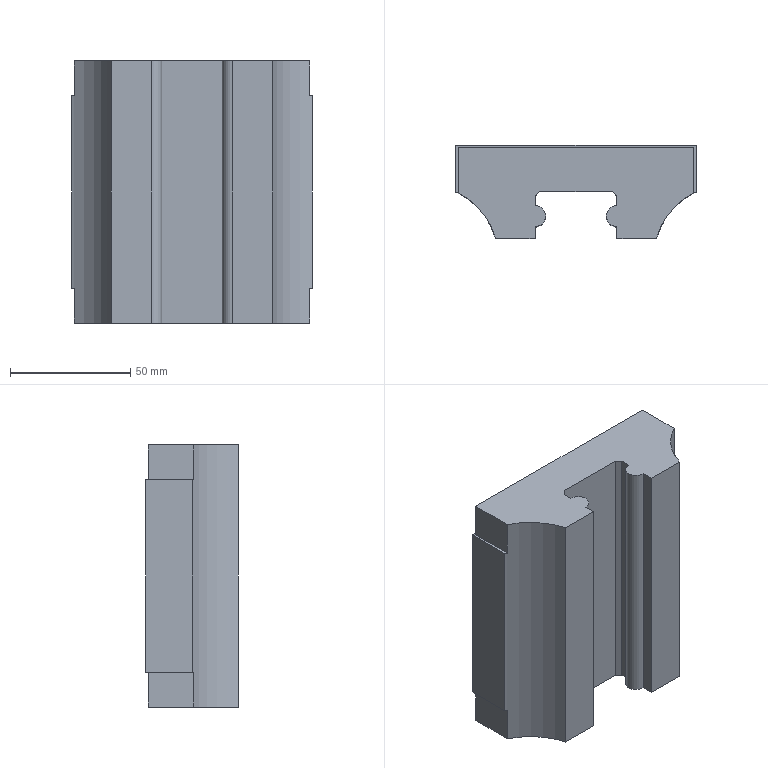Part | Creo | features CURVE 3, DATUM PLANE 3, PROTRUSION 2, COORDINATE SYSTEM 1, CUT 1 | 1 solid | 38 faces | box 100 x 38.5 x 109 mm | volume 303795 mm3 | plane 26 | cylinder 12 | commonest cylinder face diameters 6.8 x8 8.76 x2 59.72 x2
STEP:
#1=CARTESIAN_POINT('',(0.,0.,0.));
#2=DIRECTION('',(0.,0.,1.));
#3=DIRECTION('',(1.,0.,0.));
#4=AXIS2_PLACEMENT_3D('',#1,#2,#3);
#5=CARTESIAN_POINT('',(49.,37.5,-40.));
#6=VERTEX_POINT('',#5);
#7=CARTESIAN_POINT('',(-49.,37.5,-40.));
#8=VERTEX_POINT('',#7);
#9=CARTESIAN_POINT('',(49.,37.5,-40.));
#10=DIRECTION('',(-1.,0.,0.));
#11=VECTOR('',#10,98.);
#12=LINE('',#9,#11);
#13=EDGE_CURVE('',#6,#8,#12,.T.);
#14=ORIENTED_EDGE('',*,*,#13,.F.);
#15=CARTESIAN_POINT('',(49.,18.776,-40.));
#16=VERTEX_POINT('',#15);
#17=CARTESIAN_POINT('',(49.,18.776,-40.));
#18=DIRECTION('',(0.,1.,0.));
#19=VECTOR('',#18,18.724);
#20=LINE('',#17,#19);
#21=EDGE_CURVE('',#16,#6,#20,.T.);
#22=ORIENTED_EDGE('',*,*,#21,.F.);
#23=CARTESIAN_POINT('',(50.,19.25,-40.));
#24=VERTEX_POINT('',#23);
#25=CARTESIAN_POINT('',(62.277,-7.969,-40.));
#26=DIRECTION('',(0.,0.,-1.));
#27=DIRECTION('',(-0.4446,0.8957,0.));
#28=AXIS2_PLACEMENT_3D('',#25,#26,#27);
#29=CIRCLE('',#28,29.86);
#30=EDGE_CURVE('',#16,#24,#29,.T.);
#31=ORIENTED_EDGE('',*,*,#30,.T.);
#32=CARTESIAN_POINT('',(50.,38.5,-40.));
#33=VERTEX_POINT('',#32);
#34=CARTESIAN_POINT('',(50.,19.25,-40.));
#35=DIRECTION('',(0.,1.,0.));
#36=VECTOR('',#35,19.25);
#37=LINE('',#34,#36);
#38=EDGE_CURVE('',#24,#33,#37,.T.);
#39=ORIENTED_EDGE('',*,*,#38,.T.);
#40=CARTESIAN_POINT('',(-50.,38.5,-40.));
#41=VERTEX_POINT('',#40);
#42=CARTESIAN_POINT('',(50.,38.5,-40.));
#43=DIRECTION('',(-1.,0.,0.));
#44=VECTOR('',#43,100.);
#45=LINE('',#42,#44);
#46=EDGE_CURVE('',#33,#41,#45,.T.);
#47=ORIENTED_EDGE('',*,*,#46,.T.);
#48=CARTESIAN_POINT('',(-50.,19.25,-40.));
#49=VERTEX_POINT('',#48);
#50=CARTESIAN_POINT('',(-50.,38.5,-40.));
#51=DIRECTION('',(0.,-1.,0.));
#52=VECTOR('',#51,19.25);
#53=LINE('',#50,#52);
#54=EDGE_CURVE('',#41,#49,#53,.T.);
#55=ORIENTED_EDGE('',*,*,#54,.T.);
#56=CARTESIAN_POINT('',(-49.,18.776,-40.));
#57=VERTEX_POINT('',#56);
#58=CARTESIAN_POINT('',(-62.277,-7.969,-40.));
#59=DIRECTION('',(0.,0.,-1.));
#60=DIRECTION('',(0.4111,0.9116,0.));
#61=AXIS2_PLACEMENT_3D('',#58,#59,#60);
#62=CIRCLE('',#61,29.86);
#63=EDGE_CURVE('',#49,#57,#62,.T.);
#64=ORIENTED_EDGE('',*,*,#63,.T.);
#65=CARTESIAN_POINT('',(-49.,37.5,-40.));
#66=DIRECTION('',(0.,-1.,0.));
#67=VECTOR('',#66,18.724);
#68=LINE('',#65,#67);
#69=EDGE_CURVE('',#8,#57,#68,.T.);
#70=ORIENTED_EDGE('',*,*,#69,.F.);
#71=EDGE_LOOP('',(#14,#22,#31,#39,#47,#55,#64,#70));
#72=FACE_OUTER_BOUND('',#71,.F.);
#73=CARTESIAN_POINT('',(0.,0.,-40.));
#74=DIRECTION('',(0.,0.,1.));
#75=DIRECTION('',(1.,0.,0.));
#76=AXIS2_PLACEMENT_3D('',#73,#74,#75);
#77=PLANE('',#76);
#78=ADVANCED_FACE('',(#72),#77,.F.);
#79=ORIENTED_EDGE('',*,*,#13,.T.);
#80=CARTESIAN_POINT('',(-49.,37.5,-54.5));
#81=VERTEX_POINT('',#80);
#82=CARTESIAN_POINT('',(-49.,37.5,-54.5));
#83=DIRECTION('',(0.,0.,1.));
#84=VECTOR('',#83,14.5);
#85=LINE('',#82,#84);
#86=EDGE_CURVE('',#81,#8,#85,.T.);
#87=ORIENTED_EDGE('',*,*,#86,.F.);
#88=CARTESIAN_POINT('',(49.,37.5,-54.5));
#89=VERTEX_POINT('',#88);
#90=CARTESIAN_POINT('',(49.,37.5,-54.5));
#91=DIRECTION('',(-1.,0.,0.));
#92=VECTOR('',#91,98.);
#93=LINE('',#90,#92);
#94=EDGE_CURVE('',#89,#81,#93,.T.);
#95=ORIENTED_EDGE('',*,*,#94,.F.);
#96=CARTESIAN_POINT('',(49.,37.5,-54.5));
#97=DIRECTION('',(0.,0.,1.));
#98=VECTOR('',#97,14.5);
#99=LINE('',#96,#98);
#100=EDGE_CURVE('',#89,#6,#99,.T.);
#101=ORIENTED_EDGE('',*,*,#100,.T.);
#102=EDGE_LOOP('',(#79,#87,#95,#101));
#103=FACE_OUTER_BOUND('',#102,.F.);
#104=CARTESIAN_POINT('',(49.,37.5,-54.5));
#105=DIRECTION('',(0.,1.,0.));
#106=DIRECTION('',(-1.,0.,0.));
#107=AXIS2_PLACEMENT_3D('',#104,#105,#106);
#108=PLANE('',#107);
#109=ADVANCED_FACE('',(#103),#108,.T.);
#110=CARTESIAN_POINT('',(49.,37.5,40.));
#111=VERTEX_POINT('',#110);
#112=CARTESIAN_POINT('',(-49.,37.5,40.));
#113=VERTEX_POINT('',#112);
#114=CARTESIAN_POINT('',(49.,37.5,40.));
#115=DIRECTION('',(-1.,0.,0.));
#116=VECTOR('',#115,98.);
#117=LINE('',#114,#116);
#118=EDGE_CURVE('',#111,#113,#117,.T.);
#119=ORIENTED_EDGE('',*,*,#118,.F.);
#120=CARTESIAN_POINT('',(49.,37.5,54.5));
#121=VERTEX_POINT('',#120);
#122=CARTESIAN_POINT('',(49.,37.5,40.));
#123=DIRECTION('',(0.,0.,1.));
#124=VECTOR('',#123,14.5);
#125=LINE('',#122,#124);
#126=EDGE_CURVE('',#111,#121,#125,.T.);
#127=ORIENTED_EDGE('',*,*,#126,.T.);
#128=CARTESIAN_POINT('',(-49.,37.5,54.5));
#129=VERTEX_POINT('',#128);
#130=CARTESIAN_POINT('',(49.,37.5,54.5));
#131=DIRECTION('',(-1.,0.,0.));
#132=VECTOR('',#131,98.);
#133=LINE('',#130,#132);
#134=EDGE_CURVE('',#121,#129,#133,.T.);
#135=ORIENTED_EDGE('',*,*,#134,.T.);
#136=CARTESIAN_POINT('',(-49.,37.5,40.));
#137=DIRECTION('',(0.,0.,1.));
#138=VECTOR('',#137,14.5);
#139=LINE('',#136,#138);
#140=EDGE_CURVE('',#113,#129,#139,.T.);
#141=ORIENTED_EDGE('',*,*,#140,.F.);
#142=EDGE_LOOP('',(#119,#127,#135,#141));
#143=FACE_OUTER_BOUND('',#142,.F.);
#144=CARTESIAN_POINT('',(49.,37.5,-54.5));
#145=DIRECTION('',(0.,1.,0.));
#146=DIRECTION('',(-1.,0.,0.));
#147=AXIS2_PLACEMENT_3D('',#144,#145,#146);
#148=PLANE('',#147);
#149=ADVANCED_FACE('',(#143),#148,.T.);
#150=ORIENTED_EDGE('',*,*,#69,.T.);
#151=CARTESIAN_POINT('',(-49.,18.776,-54.5));
#152=VERTEX_POINT('',#151);
#153=CARTESIAN_POINT('',(-49.,18.776,-54.5));
#154=DIRECTION('',(0.,0.,1.));
#155=VECTOR('',#154,14.5);
#156=LINE('',#153,#155);
#157=EDGE_CURVE('',#152,#57,#156,.T.);
#158=ORIENTED_EDGE('',*,*,#157,.F.);
#159=CARTESIAN_POINT('',(-49.,37.5,-54.5));
#160=DIRECTION('',(0.,-1.,0.));
#161=VECTOR('',#160,18.724);
#162=LINE('',#159,#161);
#163=EDGE_CURVE('',#81,#152,#162,.T.);
#164=ORIENTED_EDGE('',*,*,#163,.F.);
#165=ORIENTED_EDGE('',*,*,#86,.T.);
#166=EDGE_LOOP('',(#150,#158,#164,#165));
#167=FACE_OUTER_BOUND('',#166,.F.);
#168=CARTESIAN_POINT('',(-49.,37.5,-54.5));
#169=DIRECTION('',(-1.,0.,0.));
#170=DIRECTION('',(0.,-1.,0.));
#171=AXIS2_PLACEMENT_3D('',#168,#169,#170);
#172=PLANE('',#171);
#173=ADVANCED_FACE('',(#167),#172,.T.);
#174=CARTESIAN_POINT('',(-49.,18.776,40.));
#175=VERTEX_POINT('',#174);
#176=CARTESIAN_POINT('',(-49.,37.5,40.));
#177=DIRECTION('',(0.,-1.,0.));
#178=VECTOR('',#177,18.724);
#179=LINE('',#176,#178);
#180=EDGE_CURVE('',#113,#175,#179,.T.);
#181=ORIENTED_EDGE('',*,*,#180,.F.);
#182=ORIENTED_EDGE('',*,*,#140,.T.);
#183=CARTESIAN_POINT('',(-49.,18.776,54.5));
#184=VERTEX_POINT('',#183);
#185=CARTESIAN_POINT('',(-49.,37.5,54.5));
#186=DIRECTION('',(0.,-1.,0.));
#187=VECTOR('',#186,18.724);
#188=LINE('',#185,#187);
#189=EDGE_CURVE('',#129,#184,#188,.T.);
#190=ORIENTED_EDGE('',*,*,#189,.T.);
#191=CARTESIAN_POINT('',(-49.,18.776,40.));
#192=DIRECTION('',(0.,0.,1.));
#193=VECTOR('',#192,14.5);
#194=LINE('',#191,#193);
#195=EDGE_CURVE('',#175,#184,#194,.T.);
#196=ORIENTED_EDGE('',*,*,#195,.F.);
#197=EDGE_LOOP('',(#181,#182,#190,#196));
#198=FACE_OUTER_BOUND('',#197,.F.);
#199=CARTESIAN_POINT('',(-49.,37.5,-54.5));
#200=DIRECTION('',(-1.,0.,0.));
#201=DIRECTION('',(0.,-1.,0.));
#202=AXIS2_PLACEMENT_3D('',#199,#200,#201);
#203=PLANE('',#202);
#204=ADVANCED_FACE('',(#198),#203,.T.);
#205=CARTESIAN_POINT('',(-50.,19.25,40.));
#206=VERTEX_POINT('',#205);
#207=CARTESIAN_POINT('',(-62.277,-7.969,40.));
#208=DIRECTION('',(0.,0.,-1.));
#209=DIRECTION('',(0.4111,0.9116,0.));
#210=AXIS2_PLACEMENT_3D('',#207,#208,#209);
#211=CIRCLE('',#210,29.86);
#212=EDGE_CURVE('',#206,#175,#211,.T.);
#213=ORIENTED_EDGE('',*,*,#212,.T.);
#214=ORIENTED_EDGE('',*,*,#195,.T.);
#215=CARTESIAN_POINT('',(-33.5,0.,54.5));
#216=VERTEX_POINT('',#215);
#217=CARTESIAN_POINT('',(-62.277,-7.969,54.5));
#218=DIRECTION('',(0.,0.,-1.));
#219=DIRECTION('',(0.4446,0.8957,0.));
#220=AXIS2_PLACEMENT_3D('',#217,#218,#219);
#221=CIRCLE('',#220,29.86);
#222=EDGE_CURVE('',#184,#216,#221,.T.);
#223=ORIENTED_EDGE('',*,*,#222,.T.);
#224=CARTESIAN_POINT('',(-33.5,0.,-54.5));
#225=VERTEX_POINT('',#224);
#226=CARTESIAN_POINT('',(-33.5,0.,-54.5));
#227=DIRECTION('',(0.,0.,1.));
#228=VECTOR('',#227,109.);
#229=LINE('',#226,#228);
#230=EDGE_CURVE('',#225,#216,#229,.T.);
#231=ORIENTED_EDGE('',*,*,#230,.F.);
#232=CARTESIAN_POINT('',(-62.277,-7.969,-54.5));
#233=DIRECTION('',(0.,0.,-1.));
#234=DIRECTION('',(0.4446,0.8957,0.));
#235=AXIS2_PLACEMENT_3D('',#232,#233,#234);
#236=CIRCLE('',#235,29.86);
#237=EDGE_CURVE('',#152,#225,#236,.T.);
#238=ORIENTED_EDGE('',*,*,#237,.F.);
#239=ORIENTED_EDGE('',*,*,#157,.T.);
#240=ORIENTED_EDGE('',*,*,#63,.F.);
#241=CARTESIAN_POINT('',(-50.,19.25,-40.));
#242=DIRECTION('',(0.,0.,1.));
#243=VECTOR('',#242,80.);
#244=LINE('',#241,#243);
#245=EDGE_CURVE('',#49,#206,#244,.T.);
#246=ORIENTED_EDGE('',*,*,#245,.T.);
#247=EDGE_LOOP('',(#213,#214,#223,#231,#238,#239,#240,#246));
#248=FACE_OUTER_BOUND('',#247,.F.);
#249=CARTESIAN_POINT('',(-62.277,-7.969,-40.));
#250=DIRECTION('',(0.,0.,1.));
#251=DIRECTION('',(1.,0.,0.));
#252=AXIS2_PLACEMENT_3D('',#249,#250,#251);
#253=CYLINDRICAL_SURFACE('',#252,29.86);
#254=ADVANCED_FACE('',(#248),#253,.F.);
#255=ORIENTED_EDGE('',*,*,#118,.T.);
#256=ORIENTED_EDGE('',*,*,#180,.T.);
#257=ORIENTED_EDGE('',*,*,#212,.F.);
#258=CARTESIAN_POINT('',(-50.,38.5,40.));
#259=VERTEX_POINT('',#258);
#260=CARTESIAN_POINT('',(-50.,38.5,40.));
#261=DIRECTION('',(0.,-1.,0.));
#262=VECTOR('',#261,19.25);
#263=LINE('',#260,#262);
#264=EDGE_CURVE('',#259,#206,#263,.T.);
#265=ORIENTED_EDGE('',*,*,#264,.F.);
#266=CARTESIAN_POINT('',(50.,38.5,40.));
#267=VERTEX_POINT('',#266);
#268=CARTESIAN_POINT('',(50.,38.5,40.));
#269=DIRECTION('',(-1.,0.,0.));
#270=VECTOR('',#269,100.);
#271=LINE('',#268,#270);
#272=EDGE_CURVE('',#267,#259,#271,.T.);
#273=ORIENTED_EDGE('',*,*,#272,.F.);
#274=CARTESIAN_POINT('',(50.,19.25,40.));
#275=VERTEX_POINT('',#274);
#276=CARTESIAN_POINT('',(50.,19.25,40.));
#277=DIRECTION('',(0.,1.,0.));
#278=VECTOR('',#277,19.25);
#279=LINE('',#276,#278);
#280=EDGE_CURVE('',#275,#267,#279,.T.);
#281=ORIENTED_EDGE('',*,*,#280,.F.);
#282=CARTESIAN_POINT('',(49.,18.776,40.));
#283=VERTEX_POINT('',#282);
#284=CARTESIAN_POINT('',(62.277,-7.969,40.));
#285=DIRECTION('',(0.,0.,-1.));
#286=DIRECTION('',(-0.4446,0.8957,0.));
#287=AXIS2_PLACEMENT_3D('',#284,#285,#286);
#288=CIRCLE('',#287,29.86);
#289=EDGE_CURVE('',#283,#275,#288,.T.);
#290=ORIENTED_EDGE('',*,*,#289,.F.);
#291=CARTESIAN_POINT('',(49.,18.776,40.));
#292=DIRECTION('',(0.,1.,0.));
#293=VECTOR('',#292,18.724);
#294=LINE('',#291,#293);
#295=EDGE_CURVE('',#283,#111,#294,.T.);
#296=ORIENTED_EDGE('',*,*,#295,.T.);
#297=EDGE_LOOP('',(#255,#256,#257,#265,#273,#281,#290,#296));
#298=FACE_OUTER_BOUND('',#297,.F.);
#299=CARTESIAN_POINT('',(0.,0.,40.));
#300=DIRECTION('',(0.,0.,1.));
#301=DIRECTION('',(1.,0.,0.));
#302=AXIS2_PLACEMENT_3D('',#299,#300,#301);
#303=PLANE('',#302);
#304=ADVANCED_FACE('',(#298),#303,.T.);
#305=ORIENTED_EDGE('',*,*,#54,.F.);
#306=CARTESIAN_POINT('',(-50.,38.5,-40.));
#307=DIRECTION('',(0.,0.,1.));
#308=VECTOR('',#307,80.);
#309=LINE('',#306,#308);
#310=EDGE_CURVE('',#41,#259,#309,.T.);
#311=ORIENTED_EDGE('',*,*,#310,.T.);
#312=ORIENTED_EDGE('',*,*,#264,.T.);
#313=ORIENTED_EDGE('',*,*,#245,.F.);
#314=EDGE_LOOP('',(#305,#311,#312,#313));
#315=FACE_OUTER_BOUND('',#314,.F.);
#316=CARTESIAN_POINT('',(-50.,38.5,-40.));
#317=DIRECTION('',(-1.,0.,0.));
#318=DIRECTION('',(0.,-1.,0.));
#319=AXIS2_PLACEMENT_3D('',#316,#317,#318);
#320=PLANE('',#319);
#321=ADVANCED_FACE('',(#315),#320,.T.);
#322=ORIENTED_EDGE('',*,*,#46,.F.);
#323=CARTESIAN_POINT('',(50.,38.5,-40.));
#324=DIRECTION('',(0.,0.,1.));
#325=VECTOR('',#324,80.);
#326=LINE('',#323,#325);
#327=EDGE_CURVE('',#33,#267,#326,.T.);
#328=ORIENTED_EDGE('',*,*,#327,.T.);
#329=ORIENTED_EDGE('',*,*,#272,.T.);
#330=ORIENTED_EDGE('',*,*,#310,.F.);
#331=EDGE_LOOP('',(#322,#328,#329,#330));
#332=FACE_OUTER_BOUND('',#331,.F.);
#333=CARTESIAN_POINT('',(44.4,38.5,-31.));
#334=VERTEX_POINT('',#333);
#335=CARTESIAN_POINT('',(37.6,38.5,-31.));
#336=VERTEX_POINT('',#335);
#337=CARTESIAN_POINT('',(41.,38.5,-31.));
#338=DIRECTION('',(0.,1.,0.));
#339=DIRECTION('',(1.,0.,0.));
#340=AXIS2_PLACEMENT_3D('',#337,#338,#339);
#341=CIRCLE('',#340,3.4);
#342=EDGE_CURVE('',#334,#336,#341,.T.);
#343=ORIENTED_EDGE('',*,*,#342,.T.);
#344=CARTESIAN_POINT('',(41.,38.5,-31.));
#345=DIRECTION('',(0.,1.,0.));
#346=DIRECTION('',(-1.,0.,0.));
#347=AXIS2_PLACEMENT_3D('',#344,#345,#346);
#348=CIRCLE('',#347,3.4);
#349=EDGE_CURVE('',#336,#334,#348,.T.);
#350=ORIENTED_EDGE('',*,*,#349,.T.);
#351=EDGE_LOOP('',(#343,#350));
#352=FACE_BOUND('',#351,.F.);
#353=CARTESIAN_POINT('',(-37.6,38.5,-31.));
#354=VERTEX_POINT('',#353);
#355=CARTESIAN_POINT('',(-44.4,38.5,-31.));
#356=VERTEX_POINT('',#355);
#357=CARTESIAN_POINT('',(-41.,38.5,-31.));
#358=DIRECTION('',(0.,1.,0.));
#359=DIRECTION('',(1.,0.,0.));
#360=AXIS2_PLACEMENT_3D('',#357,#358,#359);
#361=CIRCLE('',#360,3.4);
#362=EDGE_CURVE('',#354,#356,#361,.T.);
#363=ORIENTED_EDGE('',*,*,#362,.T.);
#364=CARTESIAN_POINT('',(-41.,38.5,-31.));
#365=DIRECTION('',(0.,1.,0.));
#366=DIRECTION('',(-1.,0.,0.));
#367=AXIS2_PLACEMENT_3D('',#364,#365,#366);
#368=CIRCLE('',#367,3.4);
#369=EDGE_CURVE('',#356,#354,#368,.T.);
#370=ORIENTED_EDGE('',*,*,#369,.T.);
#371=EDGE_LOOP('',(#363,#370));
#372=FACE_BOUND('',#371,.F.);
#373=CARTESIAN_POINT('',(-37.6,38.5,31.));
#374=VERTEX_POINT('',#373);
#375=CARTESIAN_POINT('',(-44.4,38.5,31.));
#376=VERTEX_POINT('',#375);
#377=CARTESIAN_POINT('',(-41.,38.5,31.));
#378=DIRECTION('',(0.,1.,0.));
#379=DIRECTION('',(1.,0.,0.));
#380=AXIS2_PLACEMENT_3D('',#377,#378,#379);
#381=CIRCLE('',#380,3.4);
#382=EDGE_CURVE('',#374,#376,#381,.T.);
#383=ORIENTED_EDGE('',*,*,#382,.T.);
#384=CARTESIAN_POINT('',(-41.,38.5,31.));
#385=DIRECTION('',(0.,1.,0.));
#386=DIRECTION('',(-1.,0.,0.));
#387=AXIS2_PLACEMENT_3D('',#384,#385,#386);
#388=CIRCLE('',#387,3.4);
#389=EDGE_CURVE('',#376,#374,#388,.T.);
#390=ORIENTED_EDGE('',*,*,#389,.T.);
#391=EDGE_LOOP('',(#383,#390));
#392=FACE_BOUND('',#391,.F.);
#393=CARTESIAN_POINT('',(44.4,38.5,31.));
#394=VERTEX_POINT('',#393);
#395=CARTESIAN_POINT('',(37.6,38.5,31.));
#396=VERTEX_POINT('',#395);
#397=CARTESIAN_POINT('',(41.,38.5,31.));
#398=DIRECTION('',(0.,1.,0.));
#399=DIRECTION('',(1.,0.,0.));
#400=AXIS2_PLACEMENT_3D('',#397,#398,#399);
#401=CIRCLE('',#400,3.4);
#402=EDGE_CURVE('',#394,#396,#401,.T.);
#403=ORIENTED_EDGE('',*,*,#402,.T.);
#404=CARTESIAN_POINT('',(41.,38.5,31.));
#405=DIRECTION('',(0.,1.,0.));
#406=DIRECTION('',(-1.,0.,0.));
#407=AXIS2_PLACEMENT_3D('',#404,#405,#406);
#408=CIRCLE('',#407,3.4);
#409=EDGE_CURVE('',#396,#394,#408,.T.);
#410=ORIENTED_EDGE('',*,*,#409,.T.);
#411=EDGE_LOOP('',(#403,#410));
#412=FACE_BOUND('',#411,.F.);
#413=CARTESIAN_POINT('',(50.,38.5,-40.));
#414=DIRECTION('',(0.,1.,0.));
#415=DIRECTION('',(-1.,0.,0.));
#416=AXIS2_PLACEMENT_3D('',#413,#414,#415);
#417=PLANE('',#416);
#418=ADVANCED_FACE('',(#332,#352,#372,#392,#412),#417,.T.);
#419=ORIENTED_EDGE('',*,*,#38,.F.);
#420=CARTESIAN_POINT('',(50.,19.25,-40.));
#421=DIRECTION('',(0.,0.,1.));
#422=VECTOR('',#421,80.);
#423=LINE('',#420,#422);
#424=EDGE_CURVE('',#24,#275,#423,.T.);
#425=ORIENTED_EDGE('',*,*,#424,.T.);
#426=ORIENTED_EDGE('',*,*,#280,.T.);
#427=ORIENTED_EDGE('',*,*,#327,.F.);
#428=EDGE_LOOP('',(#419,#425,#426,#427));
#429=FACE_OUTER_BOUND('',#428,.F.);
#430=CARTESIAN_POINT('',(50.,19.25,-40.));
#431=DIRECTION('',(1.,0.,0.));
#432=DIRECTION('',(0.,1.,0.));
#433=AXIS2_PLACEMENT_3D('',#430,#431,#432);
#434=PLANE('',#433);
#435=ADVANCED_FACE('',(#429),#434,.T.);
#436=CARTESIAN_POINT('',(33.5,0.,-54.5));
#437=VERTEX_POINT('',#436);
#438=CARTESIAN_POINT('',(33.5,0.,54.5));
#439=VERTEX_POINT('',#438);
#440=CARTESIAN_POINT('',(33.5,0.,-54.5));
#441=DIRECTION('',(0.,0.,1.));
#442=VECTOR('',#441,109.);
#443=LINE('',#440,#442);
#444=EDGE_CURVE('',#437,#439,#443,.T.);
#445=ORIENTED_EDGE('',*,*,#444,.T.);
#446=CARTESIAN_POINT('',(49.,18.776,54.5));
#447=VERTEX_POINT('',#446);
#448=CARTESIAN_POINT('',(62.277,-7.969,54.5));
#449=DIRECTION('',(0.,0.,-1.));
#450=DIRECTION('',(-0.9637,0.2669,0.));
#451=AXIS2_PLACEMENT_3D('',#448,#449,#450);
#452=CIRCLE('',#451,29.86);
#453=EDGE_CURVE('',#439,#447,#452,.T.);
#454=ORIENTED_EDGE('',*,*,#453,.T.);
#455=CARTESIAN_POINT('',(49.,18.776,40.));
#456=DIRECTION('',(0.,0.,1.));
#457=VECTOR('',#456,14.5);
#458=LINE('',#455,#457);
#459=EDGE_CURVE('',#283,#447,#458,.T.);
#460=ORIENTED_EDGE('',*,*,#459,.F.);
#461=ORIENTED_EDGE('',*,*,#289,.T.);
#462=ORIENTED_EDGE('',*,*,#424,.F.);
#463=ORIENTED_EDGE('',*,*,#30,.F.);
#464=CARTESIAN_POINT('',(49.,18.776,-54.5));
#465=VERTEX_POINT('',#464);
#466=CARTESIAN_POINT('',(49.,18.776,-54.5));
#467=DIRECTION('',(0.,0.,1.));
#468=VECTOR('',#467,14.5);
#469=LINE('',#466,#468);
#470=EDGE_CURVE('',#465,#16,#469,.T.);
#471=ORIENTED_EDGE('',*,*,#470,.F.);
#472=CARTESIAN_POINT('',(62.277,-7.969,-54.5));
#473=DIRECTION('',(0.,0.,-1.));
#474=DIRECTION('',(-0.9637,0.2669,0.));
#475=AXIS2_PLACEMENT_3D('',#472,#473,#474);
#476=CIRCLE('',#475,29.86);
#477=EDGE_CURVE('',#437,#465,#476,.T.);
#478=ORIENTED_EDGE('',*,*,#477,.F.);
#479=EDGE_LOOP('',(#445,#454,#460,#461,#462,#463,#471,#478));
#480=FACE_OUTER_BOUND('',#479,.F.);
#481=CARTESIAN_POINT('',(62.277,-7.969,-40.));
#482=DIRECTION('',(0.,0.,1.));
#483=DIRECTION('',(1.,0.,0.));
#484=AXIS2_PLACEMENT_3D('',#481,#482,#483);
#485=CYLINDRICAL_SURFACE('',#484,29.86);
#486=ADVANCED_FACE('',(#480),#485,.F.);
#487=CARTESIAN_POINT('',(17.,0.,-54.5));
#488=VERTEX_POINT('',#487);
#489=CARTESIAN_POINT('',(17.,0.,54.5));
#490=VERTEX_POINT('',#489);
#491=CARTESIAN_POINT('',(17.,0.,-54.5));
#492=DIRECTION('',(0.,0.,1.));
#493=VECTOR('',#492,109.);
#494=LINE('',#491,#493);
#495=EDGE_CURVE('',#488,#490,#494,.T.);
#496=ORIENTED_EDGE('',*,*,#495,.T.);
#497=CARTESIAN_POINT('',(17.,0.,54.5));
#498=DIRECTION('',(1.,0.,0.));
#499=VECTOR('',#498,16.5);
#500=LINE('',#497,#499);
#501=EDGE_CURVE('',#490,#439,#500,.T.);
#502=ORIENTED_EDGE('',*,*,#501,.T.);
#503=ORIENTED_EDGE('',*,*,#444,.F.);
#504=CARTESIAN_POINT('',(17.,0.,-54.5));
#505=DIRECTION('',(1.,0.,0.));
#506=VECTOR('',#505,16.5);
#507=LINE('',#504,#506);
#508=EDGE_CURVE('',#488,#437,#507,.T.);
#509=ORIENTED_EDGE('',*,*,#508,.F.);
#510=EDGE_LOOP('',(#496,#502,#503,#509));
#511=FACE_OUTER_BOUND('',#510,.F.);
#512=CARTESIAN_POINT('',(17.,0.,-40.));
#513=DIRECTION('',(0.,-1.,0.));
#514=DIRECTION('',(1.,0.,0.));
#515=AXIS2_PLACEMENT_3D('',#512,#513,#514);
#516=PLANE('',#515);
#517=ADVANCED_FACE('',(#511),#516,.T.);
#518=CARTESIAN_POINT('',(17.,4.72,-54.5));
#519=VERTEX_POINT('',#518);
#520=CARTESIAN_POINT('',(17.,4.72,54.5));
#521=VERTEX_POINT('',#520);
#522=CARTESIAN_POINT('',(17.,4.72,-54.5));
#523=DIRECTION('',(0.,0.,1.));
#524=VECTOR('',#523,109.);
#525=LINE('',#522,#524);
#526=EDGE_CURVE('',#519,#521,#525,.T.);
#527=ORIENTED_EDGE('',*,*,#526,.T.);
#528=CARTESIAN_POINT('',(17.,4.72,54.5));
#529=DIRECTION('',(0.,-1.,0.));
#530=VECTOR('',#529,4.72);
#531=LINE('',#528,#530);
#532=EDGE_CURVE('',#521,#490,#531,.T.);
#533=ORIENTED_EDGE('',*,*,#532,.T.);
#534=ORIENTED_EDGE('',*,*,#495,.F.);
#535=CARTESIAN_POINT('',(17.,4.72,-54.5));
#536=DIRECTION('',(0.,-1.,0.));
#537=VECTOR('',#536,4.72);
#538=LINE('',#535,#537);
#539=EDGE_CURVE('',#519,#488,#538,.T.);
#540=ORIENTED_EDGE('',*,*,#539,.F.);
#541=EDGE_LOOP('',(#527,#533,#534,#540));
#542=FACE_OUTER_BOUND('',#541,.F.);
#543=CARTESIAN_POINT('',(17.,4.72,-40.));
#544=DIRECTION('',(-1.,0.,0.));
#545=DIRECTION('',(0.,-1.,0.));
#546=AXIS2_PLACEMENT_3D('',#543,#544,#545);
#547=PLANE('',#546);
#548=ADVANCED_FACE('',(#542),#547,.T.);
#549=CARTESIAN_POINT('',(17.,13.48,-54.5));
#550=VERTEX_POINT('',#549);
#551=CARTESIAN_POINT('',(17.,13.48,54.5));
#552=VERTEX_POINT('',#551);
#553=CARTESIAN_POINT('',(17.,13.48,-54.5));
#554=DIRECTION('',(0.,0.,1.));
#555=VECTOR('',#554,109.);
#556=LINE('',#553,#555);
#557=EDGE_CURVE('',#550,#552,#556,.T.);
#558=ORIENTED_EDGE('',*,*,#557,.T.);
#559=CARTESIAN_POINT('',(17.,9.1,54.5));
#560=DIRECTION('',(0.,0.,1.));
#561=DIRECTION('',(0.,1.,0.));
#562=AXIS2_PLACEMENT_3D('',#559,#560,#561);
#563=CIRCLE('',#562,4.38);
#564=EDGE_CURVE('',#552,#521,#563,.T.);
#565=ORIENTED_EDGE('',*,*,#564,.T.);
#566=ORIENTED_EDGE('',*,*,#526,.F.);
#567=CARTESIAN_POINT('',(17.,9.1,-54.5));
#568=DIRECTION('',(0.,0.,1.));
#569=DIRECTION('',(0.,1.,0.));
#570=AXIS2_PLACEMENT_3D('',#567,#568,#569);
#571=CIRCLE('',#570,4.38);
#572=EDGE_CURVE('',#550,#519,#571,.T.);
#573=ORIENTED_EDGE('',*,*,#572,.F.);
#574=EDGE_LOOP('',(#558,#565,#566,#573));
#575=FACE_OUTER_BOUND('',#574,.F.);
#576=CARTESIAN_POINT('',(17.,9.1,-40.));
#577=DIRECTION('',(0.,0.,1.));
#578=DIRECTION('',(1.,0.,0.));
#579=AXIS2_PLACEMENT_3D('',#576,#577,#578);
#580=CYLINDRICAL_SURFACE('',#579,4.38);
#581=ADVANCED_FACE('',(#575),#580,.T.);
#582=CARTESIAN_POINT('',(17.,17.51,-54.5));
#583=VERTEX_POINT('',#582);
#584=CARTESIAN_POINT('',(17.,17.51,54.5));
#585=VERTEX_POINT('',#584);
#586=CARTESIAN_POINT('',(17.,17.51,-54.5));
#587=DIRECTION('',(0.,0.,1.));
#588=VECTOR('',#587,109.);
#589=LINE('',#586,#588);
#590=EDGE_CURVE('',#583,#585,#589,.T.);
#591=ORIENTED_EDGE('',*,*,#590,.T.);
#592=CARTESIAN_POINT('',(17.,17.51,54.5));
#593=DIRECTION('',(0.,-1.,0.));
#594=VECTOR('',#593,4.03);
#595=LINE('',#592,#594);
#596=EDGE_CURVE('',#585,#552,#595,.T.);
#597=ORIENTED_EDGE('',*,*,#596,.T.);
#598=ORIENTED_EDGE('',*,*,#557,.F.);
#599=CARTESIAN_POINT('',(17.,17.51,-54.5));
#600=DIRECTION('',(0.,-1.,0.));
#601=VECTOR('',#600,4.03);
#602=LINE('',#599,#601);
#603=EDGE_CURVE('',#583,#550,#602,.T.);
#604=ORIENTED_EDGE('',*,*,#603,.F.);
#605=EDGE_LOOP('',(#591,#597,#598,#604));
#606=FACE_OUTER_BOUND('',#605,.F.);
#607=CARTESIAN_POINT('',(17.,17.51,-40.));
#608=DIRECTION('',(-1.,0.,0.));
#609=DIRECTION('',(0.,-1.,0.));
#610=AXIS2_PLACEMENT_3D('',#607,#608,#609);
#611=PLANE('',#610);
#612=ADVANCED_FACE('',(#606),#611,.T.);
#613=CARTESIAN_POINT('',(15.,19.51,-54.5));
#614=VERTEX_POINT('',#613);
#615=CARTESIAN_POINT('',(15.,19.51,54.5));
#616=VERTEX_POINT('',#615);
#617=CARTESIAN_POINT('',(15.,19.51,-54.5));
#618=DIRECTION('',(0.,0.,1.));
#619=VECTOR('',#618,109.);
#620=LINE('',#617,#619);
#621=EDGE_CURVE('',#614,#616,#620,.T.);
#622=ORIENTED_EDGE('',*,*,#621,.T.);
#623=CARTESIAN_POINT('',(15.,19.51,54.5));
#624=DIRECTION('',(0.7071,-0.7071,0.));
#625=VECTOR('',#624,2.828);
#626=LINE('',#623,#625);
#627=EDGE_CURVE('',#616,#585,#626,.T.);
#628=ORIENTED_EDGE('',*,*,#627,.T.);
#629=ORIENTED_EDGE('',*,*,#590,.F.);
#630=CARTESIAN_POINT('',(15.,19.51,-54.5));
#631=DIRECTION('',(0.7071,-0.7071,0.));
#632=VECTOR('',#631,2.828);
#633=LINE('',#630,#632);
#634=EDGE_CURVE('',#614,#583,#633,.T.);
#635=ORIENTED_EDGE('',*,*,#634,.F.);
#636=EDGE_LOOP('',(#622,#628,#629,#635));
#637=FACE_OUTER_BOUND('',#636,.F.);
#638=CARTESIAN_POINT('',(15.,19.51,-40.));
#639=DIRECTION('',(-0.7071,-0.7071,0.));
#640=DIRECTION('',(0.7071,-0.7071,0.));
#641=AXIS2_PLACEMENT_3D('',#638,#639,#640);
#642=PLANE('',#641);
#643=ADVANCED_FACE('',(#637),#642,.T.);
#644=CARTESIAN_POINT('',(-15.,19.51,-54.5));
#645=VERTEX_POINT('',#644);
#646=CARTESIAN_POINT('',(-15.,19.51,54.5));
#647=VERTEX_POINT('',#646);
#648=CARTESIAN_POINT('',(-15.,19.51,-54.5));
#649=DIRECTION('',(0.,0.,1.));
#650=VECTOR('',#649,109.);
#651=LINE('',#648,#650);
#652=EDGE_CURVE('',#645,#647,#651,.T.);
#653=ORIENTED_EDGE('',*,*,#652,.T.);
#654=CARTESIAN_POINT('',(-15.,19.51,54.5));
#655=DIRECTION('',(1.,0.,0.));
#656=VECTOR('',#655,30.);
#657=LINE('',#654,#656);
#658=EDGE_CURVE('',#647,#616,#657,.T.);
#659=ORIENTED_EDGE('',*,*,#658,.T.);
#660=ORIENTED_EDGE('',*,*,#621,.F.);
#661=CARTESIAN_POINT('',(-15.,19.51,-54.5));
#662=DIRECTION('',(1.,0.,0.));
#663=VECTOR('',#662,30.);
#664=LINE('',#661,#663);
#665=EDGE_CURVE('',#645,#614,#664,.T.);
#666=ORIENTED_EDGE('',*,*,#665,.F.);
#667=EDGE_LOOP('',(#653,#659,#660,#666));
#668=FACE_OUTER_BOUND('',#667,.F.);
#669=CARTESIAN_POINT('',(-15.,19.51,-40.));
#670=DIRECTION('',(0.,-1.,0.));
#671=DIRECTION('',(1.,0.,0.));
#672=AXIS2_PLACEMENT_3D('',#669,#670,#671);
#673=PLANE('',#672);
#674=ADVANCED_FACE('',(#668),#673,.T.);
#675=CARTESIAN_POINT('',(-17.,17.51,-54.5));
#676=VERTEX_POINT('',#675);
#677=CARTESIAN_POINT('',(-17.,17.51,54.5));
#678=VERTEX_POINT('',#677);
#679=CARTESIAN_POINT('',(-17.,17.51,-54.5));
#680=DIRECTION('',(0.,0.,1.));
#681=VECTOR('',#680,109.);
#682=LINE('',#679,#681);
#683=EDGE_CURVE('',#676,#678,#682,.T.);
#684=ORIENTED_EDGE('',*,*,#683,.T.);
#685=CARTESIAN_POINT('',(-17.,17.51,54.5));
#686=DIRECTION('',(0.7071,0.7071,0.));
#687=VECTOR('',#686,2.828);
#688=LINE('',#685,#687);
#689=EDGE_CURVE('',#678,#647,#688,.T.);
#690=ORIENTED_EDGE('',*,*,#689,.T.);
#691=ORIENTED_EDGE('',*,*,#652,.F.);
#692=CARTESIAN_POINT('',(-17.,17.51,-54.5));
#693=DIRECTION('',(0.7071,0.7071,0.));
#694=VECTOR('',#693,2.828);
#695=LINE('',#692,#694);
#696=EDGE_CURVE('',#676,#645,#695,.T.);
#697=ORIENTED_EDGE('',*,*,#696,.F.);
#698=EDGE_LOOP('',(#684,#690,#691,#697));
#699=FACE_OUTER_BOUND('',#698,.F.);
#700=CARTESIAN_POINT('',(-17.,17.51,-40.));
#701=DIRECTION('',(0.7071,-0.7071,0.));
#702=DIRECTION('',(0.7071,0.7071,0.));
#703=AXIS2_PLACEMENT_3D('',#700,#701,#702);
#704=PLANE('',#703);
#705=ADVANCED_FACE('',(#699),#704,.T.);
#706=CARTESIAN_POINT('',(-17.,13.48,-54.5));
#707=VERTEX_POINT('',#706);
#708=CARTESIAN_POINT('',(-17.,13.48,54.5));
#709=VERTEX_POINT('',#708);
#710=CARTESIAN_POINT('',(-17.,13.48,-54.5));
#711=DIRECTION('',(0.,0.,1.));
#712=VECTOR('',#711,109.);
#713=LINE('',#710,#712);
#714=EDGE_CURVE('',#707,#709,#713,.T.);
#715=ORIENTED_EDGE('',*,*,#714,.T.);
#716=CARTESIAN_POINT('',(-17.,13.48,54.5));
#717=DIRECTION('',(0.,1.,0.));
#718=VECTOR('',#717,4.03);
#719=LINE('',#716,#718);
#720=EDGE_CURVE('',#709,#678,#719,.T.);
#721=ORIENTED_EDGE('',*,*,#720,.T.);
#722=ORIENTED_EDGE('',*,*,#683,.F.);
#723=CARTESIAN_POINT('',(-17.,13.48,-54.5));
#724=DIRECTION('',(0.,1.,0.));
#725=VECTOR('',#724,4.03);
#726=LINE('',#723,#725);
#727=EDGE_CURVE('',#707,#676,#726,.T.);
#728=ORIENTED_EDGE('',*,*,#727,.F.);
#729=EDGE_LOOP('',(#715,#721,#722,#728));
#730=FACE_OUTER_BOUND('',#729,.F.);
#731=CARTESIAN_POINT('',(-17.,13.48,-40.));
#732=DIRECTION('',(1.,0.,0.));
#733=DIRECTION('',(0.,1.,0.));
#734=AXIS2_PLACEMENT_3D('',#731,#732,#733);
#735=PLANE('',#734);
#736=ADVANCED_FACE('',(#730),#735,.T.);
#737=CARTESIAN_POINT('',(-17.,4.72,-54.5));
#738=VERTEX_POINT('',#737);
#739=CARTESIAN_POINT('',(-17.,4.72,54.5));
#740=VERTEX_POINT('',#739);
#741=CARTESIAN_POINT('',(-17.,4.72,-54.5));
#742=DIRECTION('',(0.,0.,1.));
#743=VECTOR('',#742,109.);
#744=LINE('',#741,#743);
#745=EDGE_CURVE('',#738,#740,#744,.T.);
#746=ORIENTED_EDGE('',*,*,#745,.T.);
#747=CARTESIAN_POINT('',(-17.,9.1,54.5));
#748=DIRECTION('',(0.,0.,1.));
#749=DIRECTION('',(0.,-1.,0.));
#750=AXIS2_PLACEMENT_3D('',#747,#748,#749);
#751=CIRCLE('',#750,4.38);
#752=EDGE_CURVE('',#740,#709,#751,.T.);
#753=ORIENTED_EDGE('',*,*,#752,.T.);
#754=ORIENTED_EDGE('',*,*,#714,.F.);
#755=CARTESIAN_POINT('',(-17.,9.1,-54.5));
#756=DIRECTION('',(0.,0.,1.));
#757=DIRECTION('',(0.,-1.,0.));
#758=AXIS2_PLACEMENT_3D('',#755,#756,#757);
#759=CIRCLE('',#758,4.38);
#760=EDGE_CURVE('',#738,#707,#759,.T.);
#761=ORIENTED_EDGE('',*,*,#760,.F.);
#762=EDGE_LOOP('',(#746,#753,#754,#761));
#763=FACE_OUTER_BOUND('',#762,.F.);
#764=CARTESIAN_POINT('',(-17.,9.1,-40.));
#765=DIRECTION('',(0.,0.,1.));
#766=DIRECTION('',(1.,0.,0.));
#767=AXIS2_PLACEMENT_3D('',#764,#765,#766);
#768=CYLINDRICAL_SURFACE('',#767,4.38);
#769=ADVANCED_FACE('',(#763),#768,.T.);
#770=CARTESIAN_POINT('',(-17.,0.,-54.5));
#771=VERTEX_POINT('',#770);
#772=CARTESIAN_POINT('',(-17.,0.,54.5));
#773=VERTEX_POINT('',#772);
#774=CARTESIAN_POINT('',(-17.,0.,-54.5));
#775=DIRECTION('',(0.,0.,1.));
#776=VECTOR('',#775,109.);
#777=LINE('',#774,#776);
#778=EDGE_CURVE('',#771,#773,#777,.T.);
#779=ORIENTED_EDGE('',*,*,#778,.T.);
#780=CARTESIAN_POINT('',(-17.,0.,54.5));
#781=DIRECTION('',(0.,1.,0.));
#782=VECTOR('',#781,4.72);
#783=LINE('',#780,#782);
#784=EDGE_CURVE('',#773,#740,#783,.T.);
#785=ORIENTED_EDGE('',*,*,#784,.T.);
#786=ORIENTED_EDGE('',*,*,#745,.F.);
#787=CARTESIAN_POINT('',(-17.,0.,-54.5));
#788=DIRECTION('',(0.,1.,0.));
#789=VECTOR('',#788,4.72);
#790=LINE('',#787,#789);
#791=EDGE_CURVE('',#771,#738,#790,.T.);
#792=ORIENTED_EDGE('',*,*,#791,.F.);
#793=EDGE_LOOP('',(#779,#785,#786,#792));
#794=FACE_OUTER_BOUND('',#793,.F.);
#795=CARTESIAN_POINT('',(-17.,0.,-40.));
#796=DIRECTION('',(1.,0.,0.));
#797=DIRECTION('',(0.,1.,0.));
#798=AXIS2_PLACEMENT_3D('',#795,#796,#797);
#799=PLANE('',#798);
#800=ADVANCED_FACE('',(#794),#799,.T.);
#801=ORIENTED_EDGE('',*,*,#230,.T.);
#802=CARTESIAN_POINT('',(-33.5,0.,54.5));
#803=DIRECTION('',(1.,0.,0.));
#804=VECTOR('',#803,16.5);
#805=LINE('',#802,#804);
#806=EDGE_CURVE('',#216,#773,#805,.T.);
#807=ORIENTED_EDGE('',*,*,#806,.T.);
#808=ORIENTED_EDGE('',*,*,#778,.F.);
#809=CARTESIAN_POINT('',(-33.5,0.,-54.5));
#810=DIRECTION('',(1.,0.,0.));
#811=VECTOR('',#810,16.5);
#812=LINE('',#809,#811);
#813=EDGE_CURVE('',#225,#771,#812,.T.);
#814=ORIENTED_EDGE('',*,*,#813,.F.);
#815=EDGE_LOOP('',(#801,#807,#808,#814));
#816=FACE_OUTER_BOUND('',#815,.F.);
#817=CARTESIAN_POINT('',(-33.5,0.,-40.));
#818=DIRECTION('',(0.,-1.,0.));
#819=DIRECTION('',(1.,0.,0.));
#820=AXIS2_PLACEMENT_3D('',#817,#818,#819);
#821=PLANE('',#820);
#822=ADVANCED_FACE('',(#816),#821,.T.);
#823=ORIENTED_EDGE('',*,*,#134,.F.);
#824=CARTESIAN_POINT('',(49.,18.776,54.5));
#825=DIRECTION('',(0.,1.,0.));
#826=VECTOR('',#825,18.724);
#827=LINE('',#824,#826);
#828=EDGE_CURVE('',#447,#121,#827,.T.);
#829=ORIENTED_EDGE('',*,*,#828,.F.);
#830=ORIENTED_EDGE('',*,*,#453,.F.);
#831=ORIENTED_EDGE('',*,*,#501,.F.);
#832=ORIENTED_EDGE('',*,*,#532,.F.);
#833=ORIENTED_EDGE('',*,*,#564,.F.);
#834=ORIENTED_EDGE('',*,*,#596,.F.);
#835=ORIENTED_EDGE('',*,*,#627,.F.);
#836=ORIENTED_EDGE('',*,*,#658,.F.);
#837=ORIENTED_EDGE('',*,*,#689,.F.);
#838=ORIENTED_EDGE('',*,*,#720,.F.);
#839=ORIENTED_EDGE('',*,*,#752,.F.);
#840=ORIENTED_EDGE('',*,*,#784,.F.);
#841=ORIENTED_EDGE('',*,*,#806,.F.);
#842=ORIENTED_EDGE('',*,*,#222,.F.);
#843=ORIENTED_EDGE('',*,*,#189,.F.);
#844=EDGE_LOOP('',(#823,#829,#830,#831,#832,#833,#834,#835,#836,#837,#838,#839,#840,#841,#842,#843));
#845=FACE_OUTER_BOUND('',#844,.F.);
#846=CARTESIAN_POINT('',(0.,0.,54.5));
#847=DIRECTION('',(0.,0.,1.));
#848=DIRECTION('',(1.,0.,0.));
#849=AXIS2_PLACEMENT_3D('',#846,#847,#848);
#850=PLANE('',#849);
#851=ADVANCED_FACE('',(#845),#850,.T.);
#852=ORIENTED_EDGE('',*,*,#21,.T.);
#853=ORIENTED_EDGE('',*,*,#100,.F.);
#854=CARTESIAN_POINT('',(49.,18.776,-54.5));
#855=DIRECTION('',(0.,1.,0.));
#856=VECTOR('',#855,18.724);
#857=LINE('',#854,#856);
#858=EDGE_CURVE('',#465,#89,#857,.T.);
#859=ORIENTED_EDGE('',*,*,#858,.F.);
#860=ORIENTED_EDGE('',*,*,#470,.T.);
#861=EDGE_LOOP('',(#852,#853,#859,#860));
#862=FACE_OUTER_BOUND('',#861,.F.);
#863=CARTESIAN_POINT('',(49.,18.776,-54.5));
#864=DIRECTION('',(1.,0.,0.));
#865=DIRECTION('',(0.,1.,0.));
#866=AXIS2_PLACEMENT_3D('',#863,#864,#865);
#867=PLANE('',#866);
#868=ADVANCED_FACE('',(#862),#867,.T.);
#869=ORIENTED_EDGE('',*,*,#295,.F.);
#870=ORIENTED_EDGE('',*,*,#459,.T.);
#871=ORIENTED_EDGE('',*,*,#828,.T.);
#872=ORIENTED_EDGE('',*,*,#126,.F.);
#873=EDGE_LOOP('',(#869,#870,#871,#872));
#874=FACE_OUTER_BOUND('',#873,.F.);
#875=CARTESIAN_POINT('',(49.,18.776,-54.5));
#876=DIRECTION('',(1.,0.,0.));
#877=DIRECTION('',(0.,1.,0.));
#878=AXIS2_PLACEMENT_3D('',#875,#876,#877);
#879=PLANE('',#878);
#880=ADVANCED_FACE('',(#874),#879,.T.);
#881=ORIENTED_EDGE('',*,*,#94,.T.);
#882=ORIENTED_EDGE('',*,*,#163,.T.);
#883=ORIENTED_EDGE('',*,*,#237,.T.);
#884=ORIENTED_EDGE('',*,*,#813,.T.);
#885=ORIENTED_EDGE('',*,*,#791,.T.);
#886=ORIENTED_EDGE('',*,*,#760,.T.);
#887=ORIENTED_EDGE('',*,*,#727,.T.);
#888=ORIENTED_EDGE('',*,*,#696,.T.);
#889=ORIENTED_EDGE('',*,*,#665,.T.);
#890=ORIENTED_EDGE('',*,*,#634,.T.);
#891=ORIENTED_EDGE('',*,*,#603,.T.);
#892=ORIENTED_EDGE('',*,*,#572,.T.);
#893=ORIENTED_EDGE('',*,*,#539,.T.);
#894=ORIENTED_EDGE('',*,*,#508,.T.);
#895=ORIENTED_EDGE('',*,*,#477,.T.);
#896=ORIENTED_EDGE('',*,*,#858,.T.);
#897=EDGE_LOOP('',(#881,#882,#883,#884,#885,#886,#887,#888,#889,#890,#891,#892,#893,#894,#895,#896));
#898=FACE_OUTER_BOUND('',#897,.F.);
#899=CARTESIAN_POINT('',(0.,0.,-54.5));
#900=DIRECTION('',(0.,0.,1.));
#901=DIRECTION('',(1.,0.,0.));
#902=AXIS2_PLACEMENT_3D('',#899,#900,#901);
#903=PLANE('',#902);
#904=ADVANCED_FACE('',(#898),#903,.F.);
#905=ORIENTED_EDGE('',*,*,#342,.F.);
#906=CARTESIAN_POINT('',(44.4,28.5,-31.));
#907=VERTEX_POINT('',#906);
#908=CARTESIAN_POINT('',(44.4,38.5,-31.));
#909=DIRECTION('',(0.,-1.,0.));
#910=VECTOR('',#909,10.);
#911=LINE('',#908,#910);
#912=EDGE_CURVE('',#334,#907,#911,.T.);
#913=ORIENTED_EDGE('',*,*,#912,.T.);
#914=CARTESIAN_POINT('',(37.6,28.5,-31.));
#915=VERTEX_POINT('',#914);
#916=CARTESIAN_POINT('',(41.,28.5,-31.));
#917=DIRECTION('',(0.,1.,0.));
#918=DIRECTION('',(1.,0.,0.));
#919=AXIS2_PLACEMENT_3D('',#916,#917,#918);
#920=CIRCLE('',#919,3.4);
#921=EDGE_CURVE('',#907,#915,#920,.T.);
#922=ORIENTED_EDGE('',*,*,#921,.T.);
#923=CARTESIAN_POINT('',(37.6,38.5,-31.));
#924=DIRECTION('',(0.,-1.,0.));
#925=VECTOR('',#924,10.);
#926=LINE('',#923,#925);
#927=EDGE_CURVE('',#336,#915,#926,.T.);
#928=ORIENTED_EDGE('',*,*,#927,.F.);
#929=EDGE_LOOP('',(#905,#913,#922,#928));
#930=FACE_OUTER_BOUND('',#929,.F.);
#931=CARTESIAN_POINT('',(41.,38.5,-31.));
#932=DIRECTION('',(0.,1.,0.));
#933=DIRECTION('',(1.,0.,0.));
#934=AXIS2_PLACEMENT_3D('',#931,#932,#933);
#935=CYLINDRICAL_SURFACE('',#934,3.4);
#936=ADVANCED_FACE('',(#930),#935,.F.);
#937=ORIENTED_EDGE('',*,*,#349,.F.);
#938=ORIENTED_EDGE('',*,*,#927,.T.);
#939=CARTESIAN_POINT('',(41.,28.5,-31.));
#940=DIRECTION('',(0.,1.,0.));
#941=DIRECTION('',(-1.,0.,0.));
#942=AXIS2_PLACEMENT_3D('',#939,#940,#941);
#943=CIRCLE('',#942,3.4);
#944=EDGE_CURVE('',#915,#907,#943,.T.);
#945=ORIENTED_EDGE('',*,*,#944,.T.);
#946=ORIENTED_EDGE('',*,*,#912,.F.);
#947=EDGE_LOOP('',(#937,#938,#945,#946));
#948=FACE_OUTER_BOUND('',#947,.F.);
#949=CARTESIAN_POINT('',(41.,38.5,-31.));
#950=DIRECTION('',(0.,1.,0.));
#951=DIRECTION('',(1.,0.,0.));
#952=AXIS2_PLACEMENT_3D('',#949,#950,#951);
#953=CYLINDRICAL_SURFACE('',#952,3.4);
#954=ADVANCED_FACE('',(#948),#953,.F.);
#955=ORIENTED_EDGE('',*,*,#921,.F.);
#956=ORIENTED_EDGE('',*,*,#944,.F.);
#957=EDGE_LOOP('',(#955,#956));
#958=FACE_OUTER_BOUND('',#957,.F.);
#959=CARTESIAN_POINT('',(0.,28.5,-40.));
#960=DIRECTION('',(0.,1.,0.));
#961=DIRECTION('',(1.,0.,0.));
#962=AXIS2_PLACEMENT_3D('',#959,#960,#961);
#963=PLANE('',#962);
#964=ADVANCED_FACE('',(#958),#963,.T.);
#965=CARTESIAN_POINT('',(-37.6,28.5,-31.));
#966=VERTEX_POINT('',#965);
#967=CARTESIAN_POINT('',(-44.4,28.5,-31.));
#968=VERTEX_POINT('',#967);
#969=CARTESIAN_POINT('',(-41.,28.5,-31.));
#970=DIRECTION('',(0.,1.,0.));
#971=DIRECTION('',(1.,0.,0.));
#972=AXIS2_PLACEMENT_3D('',#969,#970,#971);
#973=CIRCLE('',#972,3.4);
#974=EDGE_CURVE('',#966,#968,#973,.T.);
#975=ORIENTED_EDGE('',*,*,#974,.F.);
#976=CARTESIAN_POINT('',(-41.,28.5,-31.));
#977=DIRECTION('',(0.,1.,0.));
#978=DIRECTION('',(-1.,0.,0.));
#979=AXIS2_PLACEMENT_3D('',#976,#977,#978);
#980=CIRCLE('',#979,3.4);
#981=EDGE_CURVE('',#968,#966,#980,.T.);
#982=ORIENTED_EDGE('',*,*,#981,.F.);
#983=EDGE_LOOP('',(#975,#982));
#984=FACE_OUTER_BOUND('',#983,.F.);
#985=CARTESIAN_POINT('',(0.,28.5,-40.));
#986=DIRECTION('',(0.,1.,0.));
#987=DIRECTION('',(1.,0.,0.));
#988=AXIS2_PLACEMENT_3D('',#985,#986,#987);
#989=PLANE('',#988);
#990=ADVANCED_FACE('',(#984),#989,.T.);
#991=CARTESIAN_POINT('',(-37.6,28.5,31.));
#992=VERTEX_POINT('',#991);
#993=CARTESIAN_POINT('',(-44.4,28.5,31.));
#994=VERTEX_POINT('',#993);
#995=CARTESIAN_POINT('',(-41.,28.5,31.));
#996=DIRECTION('',(0.,1.,0.));
#997=DIRECTION('',(1.,0.,0.));
#998=AXIS2_PLACEMENT_3D('',#995,#996,#997);
#999=CIRCLE('',#998,3.4);
#1000=EDGE_CURVE('',#992,#994,#999,.T.);
#1001=ORIENTED_EDGE('',*,*,#1000,.F.);
#1002=CARTESIAN_POINT('',(-41.,28.5,31.));
#1003=DIRECTION('',(0.,1.,0.));
#1004=DIRECTION('',(-1.,0.,0.));
#1005=AXIS2_PLACEMENT_3D('',#1002,#1003,#1004);
#1006=CIRCLE('',#1005,3.4);
#1007=EDGE_CURVE('',#994,#992,#1006,.T.);
#1008=ORIENTED_EDGE('',*,*,#1007,.F.);
#1009=EDGE_LOOP('',(#1001,#1008));
#1010=FACE_OUTER_BOUND('',#1009,.F.);
#1011=CARTESIAN_POINT('',(0.,28.5,-40.));
#1012=DIRECTION('',(0.,1.,0.));
#1013=DIRECTION('',(1.,0.,0.));
#1014=AXIS2_PLACEMENT_3D('',#1011,#1012,#1013);
#1015=PLANE('',#1014);
#1016=ADVANCED_FACE('',(#1010),#1015,.T.);
#1017=CARTESIAN_POINT('',(44.4,28.5,31.));
#1018=VERTEX_POINT('',#1017);
#1019=CARTESIAN_POINT('',(37.6,28.5,31.));
#1020=VERTEX_POINT('',#1019);
#1021=CARTESIAN_POINT('',(41.,28.5,31.));
#1022=DIRECTION('',(0.,1.,0.));
#1023=DIRECTION('',(1.,0.,0.));
#1024=AXIS2_PLACEMENT_3D('',#1021,#1022,#1023);
#1025=CIRCLE('',#1024,3.4);
#1026=EDGE_CURVE('',#1018,#1020,#1025,.T.);
#1027=ORIENTED_EDGE('',*,*,#1026,.F.);
#1028=CARTESIAN_POINT('',(41.,28.5,31.));
#1029=DIRECTION('',(0.,1.,0.));
#1030=DIRECTION('',(-1.,0.,0.));
#1031=AXIS2_PLACEMENT_3D('',#1028,#1029,#1030);
#1032=CIRCLE('',#1031,3.4);
#1033=EDGE_CURVE('',#1020,#1018,#1032,.T.);
#1034=ORIENTED_EDGE('',*,*,#1033,.F.);
#1035=EDGE_LOOP('',(#1027,#1034));
#1036=FACE_OUTER_BOUND('',#1035,.F.);
#1037=CARTESIAN_POINT('',(0.,28.5,-40.));
#1038=DIRECTION('',(0.,1.,0.));
#1039=DIRECTION('',(1.,0.,0.));
#1040=AXIS2_PLACEMENT_3D('',#1037,#1038,#1039);
#1041=PLANE('',#1040);
#1042=ADVANCED_FACE('',(#1036),#1041,.T.);
#1043=ORIENTED_EDGE('',*,*,#362,.F.);
#1044=CARTESIAN_POINT('',(-37.6,38.5,-31.));
#1045=DIRECTION('',(0.,-1.,0.));
#1046=VECTOR('',#1045,10.);
#1047=LINE('',#1044,#1046);
#1048=EDGE_CURVE('',#354,#966,#1047,.T.);
#1049=ORIENTED_EDGE('',*,*,#1048,.T.);
#1050=ORIENTED_EDGE('',*,*,#974,.T.);
#1051=CARTESIAN_POINT('',(-44.4,38.5,-31.));
#1052=DIRECTION('',(0.,-1.,0.));
#1053=VECTOR('',#1052,10.);
#1054=LINE('',#1051,#1053);
#1055=EDGE_CURVE('',#356,#968,#1054,.T.);
#1056=ORIENTED_EDGE('',*,*,#1055,.F.);
#1057=EDGE_LOOP('',(#1043,#1049,#1050,#1056));
#1058=FACE_OUTER_BOUND('',#1057,.F.);
#1059=CARTESIAN_POINT('',(-41.,38.5,-31.));
#1060=DIRECTION('',(0.,1.,0.));
#1061=DIRECTION('',(1.,0.,0.));
#1062=AXIS2_PLACEMENT_3D('',#1059,#1060,#1061);
#1063=CYLINDRICAL_SURFACE('',#1062,3.4);
#1064=ADVANCED_FACE('',(#1058),#1063,.F.);
#1065=ORIENTED_EDGE('',*,*,#369,.F.);
#1066=ORIENTED_EDGE('',*,*,#1055,.T.);
#1067=ORIENTED_EDGE('',*,*,#981,.T.);
#1068=ORIENTED_EDGE('',*,*,#1048,.F.);
#1069=EDGE_LOOP('',(#1065,#1066,#1067,#1068));
#1070=FACE_OUTER_BOUND('',#1069,.F.);
#1071=CARTESIAN_POINT('',(-41.,38.5,-31.));
#1072=DIRECTION('',(0.,1.,0.));
#1073=DIRECTION('',(1.,0.,0.));
#1074=AXIS2_PLACEMENT_3D('',#1071,#1072,#1073);
#1075=CYLINDRICAL_SURFACE('',#1074,3.4);
#1076=ADVANCED_FACE('',(#1070),#1075,.F.);
#1077=ORIENTED_EDGE('',*,*,#382,.F.);
#1078=CARTESIAN_POINT('',(-37.6,38.5,31.));
#1079=DIRECTION('',(0.,-1.,0.));
#1080=VECTOR('',#1079,10.);
#1081=LINE('',#1078,#1080);
#1082=EDGE_CURVE('',#374,#992,#1081,.T.);
#1083=ORIENTED_EDGE('',*,*,#1082,.T.);
#1084=ORIENTED_EDGE('',*,*,#1000,.T.);
#1085=CARTESIAN_POINT('',(-44.4,38.5,31.));
#1086=DIRECTION('',(0.,-1.,0.));
#1087=VECTOR('',#1086,10.);
#1088=LINE('',#1085,#1087);
#1089=EDGE_CURVE('',#376,#994,#1088,.T.);
#1090=ORIENTED_EDGE('',*,*,#1089,.F.);
#1091=EDGE_LOOP('',(#1077,#1083,#1084,#1090));
#1092=FACE_OUTER_BOUND('',#1091,.F.);
#1093=CARTESIAN_POINT('',(-41.,38.5,31.));
#1094=DIRECTION('',(0.,1.,0.));
#1095=DIRECTION('',(1.,0.,0.));
#1096=AXIS2_PLACEMENT_3D('',#1093,#1094,#1095);
#1097=CYLINDRICAL_SURFACE('',#1096,3.4);
#1098=ADVANCED_FACE('',(#1092),#1097,.F.);
#1099=ORIENTED_EDGE('',*,*,#389,.F.);
#1100=ORIENTED_EDGE('',*,*,#1089,.T.);
#1101=ORIENTED_EDGE('',*,*,#1007,.T.);
#1102=ORIENTED_EDGE('',*,*,#1082,.F.);
#1103=EDGE_LOOP('',(#1099,#1100,#1101,#1102));
#1104=FACE_OUTER_BOUND('',#1103,.F.);
#1105=CARTESIAN_POINT('',(-41.,38.5,31.));
#1106=DIRECTION('',(0.,1.,0.));
#1107=DIRECTION('',(1.,0.,0.));
#1108=AXIS2_PLACEMENT_3D('',#1105,#1106,#1107);
#1109=CYLINDRICAL_SURFACE('',#1108,3.4);
#1110=ADVANCED_FACE('',(#1104),#1109,.F.);
#1111=ORIENTED_EDGE('',*,*,#402,.F.);
#1112=CARTESIAN_POINT('',(44.4,38.5,31.));
#1113=DIRECTION('',(0.,-1.,0.));
#1114=VECTOR('',#1113,10.);
#1115=LINE('',#1112,#1114);
#1116=EDGE_CURVE('',#394,#1018,#1115,.T.);
#1117=ORIENTED_EDGE('',*,*,#1116,.T.);
#1118=ORIENTED_EDGE('',*,*,#1026,.T.);
#1119=CARTESIAN_POINT('',(37.6,38.5,31.));
#1120=DIRECTION('',(0.,-1.,0.));
#1121=VECTOR('',#1120,10.);
#1122=LINE('',#1119,#1121);
#1123=EDGE_CURVE('',#396,#1020,#1122,.T.);
#1124=ORIENTED_EDGE('',*,*,#1123,.F.);
#1125=EDGE_LOOP('',(#1111,#1117,#1118,#1124));
#1126=FACE_OUTER_BOUND('',#1125,.F.);
#1127=CARTESIAN_POINT('',(41.,38.5,31.));
#1128=DIRECTION('',(0.,1.,0.));
#1129=DIRECTION('',(1.,0.,0.));
#1130=AXIS2_PLACEMENT_3D('',#1127,#1128,#1129);
#1131=CYLINDRICAL_SURFACE('',#1130,3.4);
#1132=ADVANCED_FACE('',(#1126),#1131,.F.);
#1133=ORIENTED_EDGE('',*,*,#409,.F.);
#1134=ORIENTED_EDGE('',*,*,#1123,.T.);
#1135=ORIENTED_EDGE('',*,*,#1033,.T.);
#1136=ORIENTED_EDGE('',*,*,#1116,.F.);
#1137=EDGE_LOOP('',(#1133,#1134,#1135,#1136));
#1138=FACE_OUTER_BOUND('',#1137,.F.);
#1139=CARTESIAN_POINT('',(41.,38.5,31.));
#1140=DIRECTION('',(0.,1.,0.));
#1141=DIRECTION('',(1.,0.,0.));
#1142=AXIS2_PLACEMENT_3D('',#1139,#1140,#1141);
#1143=CYLINDRICAL_SURFACE('',#1142,3.4);
#1144=ADVANCED_FACE('',(#1138),#1143,.F.);
#1145=CLOSED_SHELL('',(#78,#109,#149,#173,#204,#254,#304,#321,#418,#435,#486,#517,#548,#581,#612,#643,#674,#705,#736,#769,#800,#822,#851,#868,#880,#904,#936,#954,#964,#990,#1016,#1042,#1064,#1076,#1098,#1110,#1132,#1144));
#1146=MANIFOLD_SOLID_BREP('',#1145);
#1147=(LENGTH_UNIT()NAMED_UNIT(*)SI_UNIT(.MILLI.,.METRE.));
#1148=UNCERTAINTY_MEASURE_WITH_UNIT(LENGTH_MEASURE(0.01528),#1147,'','');
#1149=(NAMED_UNIT(*)PLANE_ANGLE_UNIT()SI_UNIT($,.RADIAN.));
#1150=PLANE_ANGLE_MEASURE_WITH_UNIT(PLANE_ANGLE_MEASURE(0.01745),#1149);
#1151=(CONVERSION_BASED_UNIT('DEGREE',#1150)NAMED_UNIT(*)PLANE_ANGLE_UNIT());
#1152=(NAMED_UNIT(*)SI_UNIT($,.STERADIAN.)SOLID_ANGLE_UNIT());
#1153=(GEOMETRIC_REPRESENTATION_CONTEXT(3)GLOBAL_UNCERTAINTY_ASSIGNED_CONTEXT((#1148))GLOBAL_UNIT_ASSIGNED_CONTEXT((#1147,#1151,#1152))REPRESENTATION_CONTEXT('',''));
#1154=ADVANCED_BREP_SHAPE_REPRESENTATION('',(#4,#1146),#1153);